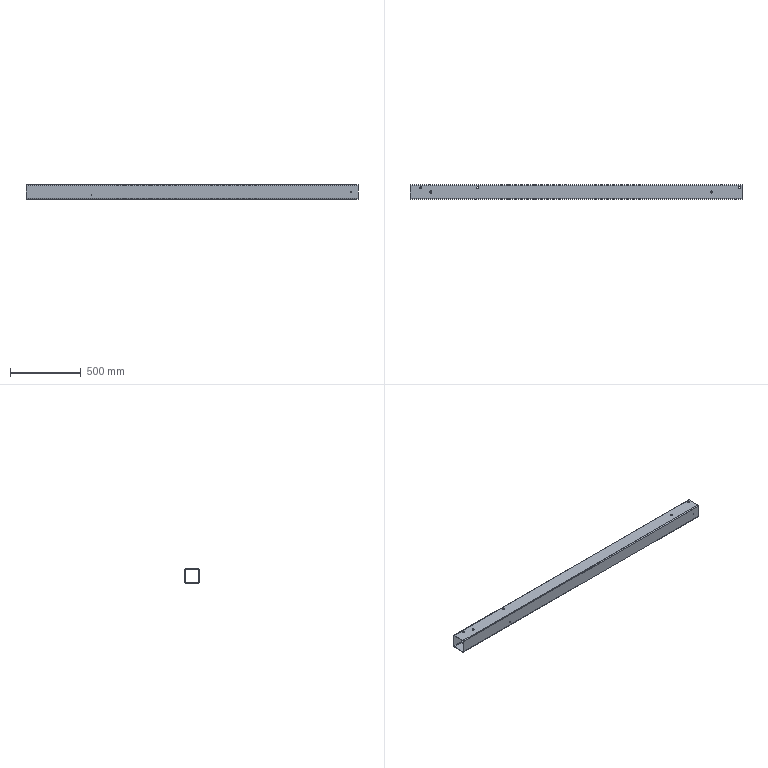Part | STEP file | [01] | 1 solid | 48 faces | box 2349 x 100 x 100 mm | volume 2841640 mm3 | cylinder 38 | plane 10 | commonest cylinder face diameters 15 x20 12 x6 6 x4 6.4 x4 12.8 x4